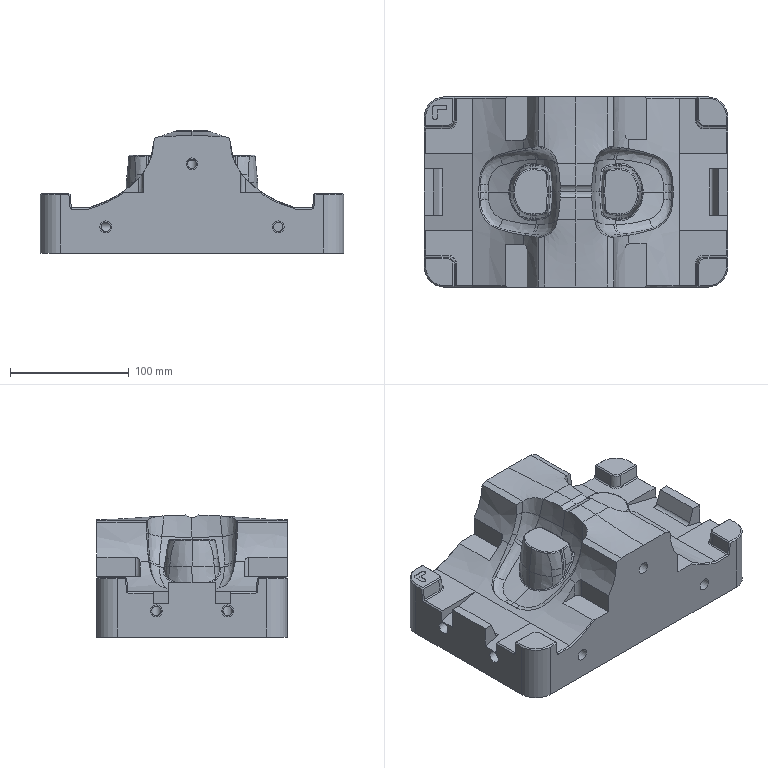NC program | NX | posted with a generic post | part box 255 x 160 x 102.619 mm
Lines 31654 to 32439 of 55104:
(ZLEVEL_PROFILE , TOOL : D8)
N63276 M6
N63278 G54
N63280 G17 G0 G90 X145.704 Y78.046 S3000 M3
N63282 G43 Z102.821 H0
N63284 G94 G1 Z102.321 F1800.
N63286 G3 X144.835 Y75.38 R4.
N63288 X145.715 Y64.863 R130.417
N63290 G1 X145.758 Y64.534 Z102.303
N63292 X145.803 Y64.205 Z102.286
N63294 X145.848 Y63.876 Z102.268
N63296 X145.894 Y63.547 Z102.25
N63298 X145.942 Y63.218 Z102.233
N63300 X145.99 Y62.889 Z102.215
N63302 X146.038 Y62.56 Z102.198
N63304 X146.139 Y61.903 Z102.163
N63306 X146.19 Y61.575 Z102.145
N63308 X146.243 Y61.246 Z102.127
N63310 X146.297 Y60.918 Z102.11
N63312 X146.351 Y60.59 Z102.092
N63314 X146.406 Y60.263 Z102.075
N63316 X146.463 Y59.935 Z102.057
N63318 X146.519 Y59.608 Z102.039
N63320 X146.576 Y59.28 Z102.022
N63322 G2 X144.847 Y75.699 R125.065
N63324 G1 X144.858 Y75.884 Z101.872
N63326 X144.854 Y76.068 Z101.723
N63328 G3 X146.596 Y59.289 R129.197
N63330 X147.378 Y55.437 R51.336
N63332 G1 Z103.723
N63334 G0 X147.537 Y97.962 Z102.821
N63336 G1 Z102.321
N63338 G3 X145.706 Y95.075 R4.
N63340 X144.836 Y84.633 R129.482
N63342 G1 X144.847 Y84.307 Z102.022
N63344 G2 X146.578 Y100.732 R124.772
N63346 G1 X146.636 Y101.053 Z101.997
N63348 X146.695 Y101.374 Z101.972
N63350 X146.755 Y101.694 Z101.947
N63352 X146.816 Y102.015 Z101.922
N63354 X146.878 Y102.336 Z101.897
N63356 X146.94 Y102.656 Z101.872
N63358 X147.005 Y102.976 Z101.847
N63360 X147.073 Y103.295 Z101.823
N63362 X147.144 Y103.614 Z101.798
N63364 X147.22 Y103.932 Z101.773
N63366 X147.3 Y104.248 Z101.748
N63368 X147.378 Y104.565 Z101.723
N63370 G3 X146.367 Y99.334 R63.16
N63372 G1 X146.151 Y97.953
N63374 G3 X144.853 Y83.935 R132.505
N63376 G1 Z103.723
N63378 G0 X150.199 Y51.086 Z101.924
N63380 G1 Z101.424
N63382 G2 X148.113 Y53.287 R4.
N63384 X147.001 Y57.217 R21.719
N63386 X144.87 Y76.489 R123.807
N63388 G3 X142.79 Y80.002 R4.184
N63390 X144.871 Y83.514 R4.196
N63392 G2 X147.001 Y102.786 R123.362
N63394 X148.115 Y106.72 R21.686
N63396 G1 X148.247 Y107.019 Z101.364
N63398 X148.381 Y107.318 Z101.304
N63400 X148.522 Y107.613 Z101.245
N63402 X148.67 Y107.906 Z101.185
N63404 X148.818 Y108.198 Z101.125
N63406 G3 X147.087 Y103.111 R19.726
N63408 X144.882 Y82.989 R123.078
N63410 G2 X143.554 Y80.002 R4.202
N63412 X144.882 Y77.009 R4.199
N63414 G3 X147.077 Y56.94 R123.912
N63416 X148.821 Y51.801 R19.921
N63418 G1 X148.985 Y51.522 Z101.05
N63420 X149.152 Y51.244 Z100.975
N63422 X149.327 Y50.97 Z100.901
N63424 X149.506 Y50.699 Z100.826
N63426 G2 X147.183 Y56.527 R16.935
N63428 X144.888 Y77.68 R123.758
N63430 G3 X144.196 Y80.002 R4.49
N63432 X144.888 Y82.321 R4.476
N63434 G2 X147.183 Y103.476 R123.252
N63436 X149.506 Y109.305 R16.932
N63438 G1 X149.664 Y109.523 Z100.751
N63440 X149.825 Y109.738 Z100.677
N63442 X149.992 Y109.95 Z100.602
N63444 X150.16 Y110.16 Z100.527
N63446 G3 X147.874 Y105.899 R13.8
N63448 X147.041 Y102.654 R25.809
N63450 X144.901 Y81.324 R124.227
N63452 G2 X144.753 Y80.002 R5.63
N63454 X144.901 Y78.679 R5.664
N63456 G3 X147.204 Y56.527 R123.237
N63458 X149.019 Y51.526 R17.978
N63460 X150.161 Y49.841 R10.25
N63462 G1 X150.377 Y49.605 Z100.427
N63464 X150.595 Y49.371 Z100.328
N63466 X150.817 Y49.141 Z100.228
N63468 G2 X148.571 Y52.428 R12.025
N63470 X147.179 Y56.771 R18.625
N63472 G1 X147.095 Y57.217
N63474 G2 X147.095 Y102.786 R121.14
N63476 G1 X147.141 Y103.029
N63478 G2 X148.309 Y106.987 R20.755
N63480 X150.817 Y110.863 R12.366
N63482 G1 X151.032 Y111.062 Z100.128
N63484 X151.249 Y111.259 Z100.029
N63486 X151.47 Y111.451 Z99.929
N63488 G3 X148.611 Y107.619 R11.659
N63490 X147.293 Y103.695 R19.539
N63492 X147.118 Y57.217 R121.302
N63494 G1 X147.188 Y56.841
N63496 G3 X148.599 Y52.41 R18.833
N63498 X151.47 Y48.552 R11.664
N63500 G1 X151.689 Y48.378 Z99.829
N63502 X151.91 Y48.208 Z99.73
N63504 X152.136 Y48.043 Z99.63
N63506 G2 X148.622 Y52.404 R11.441
N63508 X147.2 Y56.902 R18.959
N63510 G1 X147.142 Y57.217
N63512 G2 X146.973 Y101.869 R121.296
N63514 G1 X147.2 Y103.101
N63516 G2 X148.623 Y107.602 R18.929
N63518 X152.136 Y111.96 R11.447
N63520 G1 X152.348 Y112.105 Z99.53
N63522 X152.563 Y112.245 Z99.431
N63524 X152.78 Y112.382 Z99.331
N63526 G3 X148.673 Y107.666 R11.319
N63528 X147.29 Y103.476 R19.849
N63530 G1 X146.936 Y101.516
N63532 G3 X147.165 Y57.217 R121.39
N63534 G1 X147.293 Y56.511
N63536 G3 X148.673 Y52.338 R19.835
N63538 X152.776 Y47.624 R11.32
N63540 G1 X152.998 Y47.495 Z99.232
N63542 X153.222 Y47.37 Z99.132
N63544 X153.448 Y47.249 Z99.032
N63546 G2 X148.564 Y52.62 R11.269
N63548 X147.272 Y56.782 R20.026
N63550 X146.956 Y101.493 R121.596
N63552 G1 X147.246 Y103.106
N63554 G2 X148.676 Y107.632 R18.565
N63556 X153.445 Y112.752 R11.268
N63558 G1 X153.67 Y112.866 Z98.933
N63560 X153.898 Y112.976 Z98.833
N63562 X154.127 Y113.084 Z98.733
N63564 G3 X148.673 Y107.577 R11.28
N63566 X147.344 Y103.476 R18.726
N63568 X147.344 Y56.527 R122.248
N63570 X148.673 Y52.426 R19.026
N63572 X154.123 Y46.921 R11.279
N63574 G1 X154.355 Y46.822 Z98.634
N63576 X154.588 Y46.725 Z98.534
N63578 X154.821 Y46.629 Z98.434
N63580 G2 X148.673 Y52.476 R11.373
N63582 X147.372 Y56.527 R18.468
N63584 X147.372 Y103.476 R122.212
N63586 X148.673 Y107.527 R18.518
N63588 X154.818 Y113.373 R11.371
N63590 G1 Z100.434
N63592 G0 X159.396 Y162.579 Z98.635
N63594 G1 Z98.135
N63596 G3 X158.453 Y160.001 R4.
N63598 G1 X158.443 Y117.702
N63600 G2 X155.472 Y113.594 R4.327
N63602 G3 X148.673 Y107.477 R11.373
N63604 X147.399 Y103.476 R17.602
N63606 X147.4 Y56.527 R122.194
N63608 X149.709 Y50.694 R15.93
N63610 X155.365 Y46.445 R11.47
N63612 G2 X157.52 Y45. R5.05
N63614 X158.454 Y42.52 R3.759
N63616 G1 X158.453 Y0.002
N63618 X158.901 Z97.986
N63620 X159.346 Z97.836
N63622 X159.347 Y42.028
N63624 G3 X156.266 Y46.148 R4.19
N63626 G2 X153.704 Y47.201 R16.024
N63628 X149.137 Y51.675 R10.864
N63630 X147.427 Y56.527 R16.322
N63632 X147.427 Y103.476 R122.318
N63634 X148.77 Y107.619 R16.963
N63636 X152.063 Y111.761 R11.209
N63638 X156.266 Y113.849 R13.589
N63640 G3 X159.347 Y117.975 R4.205
N63642 G1 X159.346 Y160.001
N63644 X159.794 Z97.687
N63646 X160.24 Z97.537
N63648 X160.241 Y118.666
N63650 X160.24 Y117.975
N63652 G2 X156.956 Y114.025 R4.237
N63654 G3 X152.709 Y112.184 R14.04
N63656 X149.128 Y108.281 R10.542
N63658 X147.455 Y103.476 R16.685
N63660 X147.455 Y56.527 R122.482
N63662 X149.117 Y51.752 R16.366
N63664 X154.113 Y47.019 R10.863
N63666 X157.223 Y45.879 R19.541
N63668 G2 X160.24 Y41.929 R4.095
N63670 G1 Y0.002
N63672 X160.688 Z97.388
N63674 X161.134 Z97.238
N63676 X161.135 Y41.337
N63678 X161.126 Y42.028
N63680 G3 X157.668 Y45.825 R4.232
N63682 G2 X153.73 Y47.236 R15.521
N63684 X149.042 Y51.935 R10.962
N63686 X147.625 Y55.836 R16.256
N63688 G1 X147.342 Y57.217
N63690 G2 X147.482 Y103.476 R122.922
N63692 X149.118 Y108.212 R16.513
N63694 X153.054 Y112.377 R10.661
N63696 X157.68 Y114.178 R14.627
N63698 G3 X161.126 Y117.975 R4.245
N63700 G1 X161.135 Y118.666
N63702 X161.134 Y160.001
N63704 X161.582 Z97.089
N63706 X162.028 Z96.939
N63708 X162.029 Y118.666
N63710 X162.019 Y118.32
N63712 G2 X158.472 Y114.309 R4.183
N63714 G3 X153.043 Y112.347 R14.921
N63716 X149.168 Y108.258 R10.537
N63718 X147.51 Y103.476 R16.458
N63720 X147.51 Y56.527 R122.96
N63722 X149.083 Y51.907 R16.32
N63724 X153.808 Y47.218 R10.88
N63726 X158.523 Y45.676 R16.092
N63728 G2 X162.029 Y41.553 R4.177
N63730 G1 X162.028 Y0.002
N63732 X162.476 Z96.79
N63734 X162.915 Z96.64
N63736 X162.916 Y41.473
N63738 G3 X159.251 Y45.592 R4.147
N63740 G2 X153.844 Y47.222 R16.097
N63742 X149.088 Y51.949 R10.883
N63744 X147.538 Y56.527 R16.295
N63746 X147.538 Y103.476 R123.304
N63748 X149.164 Y108.206 R16.549
N63750 X153.067 Y112.337 R10.503
N63752 X158.336 Y114.271 R15.004
N63754 G1 X159.026 Y114.374
N63756 X159.533 Y114.464
N63758 G3 X162.916 Y118.505 R4.105
N63760 G1 X162.915 Y160.001
N63762 X163.018 Z96.603
N63764 X163.143 Z96.566
N63766 X163.184 Z96.528
N63768 X163.206 Z96.491
N63770 X163.22 Z96.342
N63772 X163.221 Y118.473
N63774 G2 X159.547 Y114.425 R4.067
N63776 G3 X153.538 Y112.591 R15.857
N63778 X149.149 Y108.127 R10.65
N63780 X147.565 Y103.476 R16.401
N63782 X147.566 Y56.527 R123.661
N63784 G1 X147.713 Y55.836
N63786 G3 X149.41 Y51.419 R14.926
N63788 X153.816 Y47.255 R10.683
N63790 X159.561 Y45.575 R16.266
N63792 G2 X163.221 Y41.532 R4.063
N63794 G1 X163.22 Y0.002
N63796 X163.24 Z96.043
N63798 Y41.542
N63800 G3 X159.568 Y45.593 R4.071
N63802 G2 X153.801 Y47.287 R16.104
N63804 X149.384 Y51.507 R10.715
N63806 X147.744 Y55.836 R14.786
N63808 G1 X147.593 Y56.527
N63810 G2 X147.593 Y103.476 R124.031
N63812 X148.922 Y107.619 R16.478
N63814 X153.962 Y112.797 R10.835
N63816 X159.567 Y114.41 R16.083
N63818 G3 X163.241 Y118.463 R4.072
N63820 G1 X163.24 Y160.001
N63822 X163.261 Z95.744
N63824 X163.262 Y118.451
N63826 G2 X159.581 Y114.396 R4.074
N63828 G3 X153.373 Y112.452 R15.824
N63830 X148.947 Y107.619 R10.749
N63832 X147.621 Y103.476 R17.174
N63834 G1 X147.251 Y101.375
N63836 G3 X147.499 Y57.217 R123.536
N63838 G1 X147.621 Y56.527
N63840 G3 X148.947 Y52.384 R17.143
N63842 X154.01 Y47.206 R10.831
N63844 X159.566 Y45.609 R16.14
N63846 G2 X163.261 Y41.524 R4.105
N63848 G1 X163.26 Y0.002
N63850 X163.282 Z95.445
N63852 X163.283 Y41.534
N63854 G3 X159.585 Y45.622 R4.109
N63856 G2 X154.059 Y47.206 R16.142
N63858 X148.972 Y52.384 R10.858
N63860 X147.651 Y56.527 R17.345
N63862 G1 X147.531 Y57.217
N63864 G2 X147.258 Y101.22 R123.691
N63866 G1 X147.651 Y103.476
N63868 G2 X148.972 Y107.619 R17.416
N63870 X153.417 Y112.452 R10.786
N63872 X159.603 Y114.383 R15.869
N63874 G3 X163.284 Y118.44 R4.076
N63876 G1 X163.283 Y160.001
N63878 X163.304 Z95.146
N63880 X163.306 Y118.427
N63882 G2 X159.626 Y114.37 R4.076
N63884 G3 X153.461 Y112.452 R15.91
N63886 X148.997 Y107.619 R10.827
N63888 X147.686 Y103.476 R17.336
N63890 X147.687 Y56.527 R124.646
N63892 X149.097 Y52.195 R16.412
N63894 X153.918 Y47.301 R10.798
N63896 X159.608 Y45.635 R16.161
N63898 G2 X163.305 Y41.547 R4.108
N63900 G1 X163.304 Y0.002
N63902 X163.326 Z94.847
N63904 X163.327 Y41.561
N63906 G3 X159.627 Y45.648 R4.107
N63908 G2 X153.607 Y47.495 R15.979
N63910 X149.197 Y52.05 R10.538
N63912 X147.722 Y56.527 R16.282
N63914 X147.721 Y103.476 R124.68
N63916 X149.024 Y107.619 R17.379
N63918 X153.505 Y112.452 R10.863
N63920 X159.626 Y114.355 R15.974
N63922 G3 X163.328 Y118.443 R4.109
N63924 G1 X163.326 Y160.001
N63926 X163.35 Z94.548
N63928 X163.352 Y118.431
N63930 G2 X159.651 Y114.342 R4.109
N63932 G3 X153.555 Y112.452 R15.957
N63934 X149.056 Y107.619 R10.792
N63936 X147.757 Y103.476 R16.978
N63938 X147.757 Y56.527 R124.676
N63940 G1 X147.9 Y55.836
N63942 G3 X149.364 Y51.785 R15.403
N63944 X153.85 Y47.399 R10.668
N63946 X159.648 Y45.661 R15.823
N63948 G2 X163.35 Y41.574 R4.107
N63950 G1 Y0.002
N63952 X163.377 Z94.249
N63954 Y41.614
N63956 G3 X159.704 Y45.672 R4.078
N63958 G2 X153.953 Y47.362 R16.184
N63960 X149.218 Y52.135 R10.772
N63962 X147.931 Y55.836 R15.189
N63964 X147.931 Y104.167 R124.532
N63966 X149.089 Y107.619 R16.017
N63968 X153.606 Y112.452 R10.732
N63970 X159.679 Y114.33 R15.995
N63972 G3 X163.378 Y118.419 R4.11
N63974 G1 X163.377 Y160.001
N63976 X163.403 Z93.95
N63978 X163.405 Y118.379
N63980 G2 X159.731 Y114.319 R4.079
N63982 G3 X153.657 Y112.452 R16.079
N63984 X149.122 Y107.619 R10.672
N63986 X147.962 Y104.167 R15.519
N63988 X147.962 Y55.836 R125.019
N63990 X149.48 Y51.694 R14.914
N63992 X154.195 Y47.269 R10.714
N63994 X159.73 Y45.685 R16.138
N63996 G2 X163.404 Y41.626 R4.079
N63998 G1 X163.403 Y0.002
N64000 X163.43 Z93.651
N64002 X163.431 Y41.637
N64004 G3 X159.753 Y45.699 R4.082
N64006 G2 X153.709 Y47.551 R16.046
N64008 X149.364 Y51.96 R10.647
N64010 X147.995 Y55.836 R15.525
N64012 X147.995 Y104.167 R125.489
N64014 X149.154 Y107.619 R15.665
N64016 X153.709 Y112.452 R10.63
N64018 X159.76 Y114.307 R16.126
N64020 G3 X163.432 Y118.366 R4.079
N64022 G1 X163.43 Y160.001
N64024 X163.457 Z93.352
N64026 X163.458 Y118.354
N64028 G2 X159.779 Y114.293 R4.08
N64030 G3 X153.505 Y112.301 R15.876
N64032 X149.187 Y107.619 R10.489
N64034 X148.033 Y104.167 R15.649
N64036 X148.033 Y55.836 R125.594
N64038 X149.364 Y52.018 R15.682
N64040 X153.505 Y47.702 R10.521
N64042 X159.773 Y45.713 R15.821
N64044 G2 X163.457 Y41.649 R4.083
N64046 G1 Y0.002
N64048 X163.483 Z93.053
N64050 X163.484 Y41.661
N64052 G3 X159.8 Y45.726 R4.084
N64054 G2 X153.505 Y47.732 R15.807
N64056 X149.182 Y52.458 R10.488
N64058 X148.02 Y56.074 R15.919
N64060 X148.071 Y104.167 R125.7
N64062 X149.219 Y107.619 R15.404
N64064 X153.505 Y112.271 R10.457
N64066 X159.805 Y114.28 R15.868
N64068 G3 X163.485 Y118.343 R4.082
N64070 G1 X163.483 Y160.001
N64072 X163.51 Z92.754
N64074 X163.512 Y118.331
N64076 G2 X159.831 Y114.267 R4.084
N64078 G3 X153.505 Y112.241 R15.859
N64080 X149.252 Y107.619 R10.457
N64082 X148.108 Y104.167 R15.197
N64084 X148.108 Y55.836 R125.772
N64086 X149.364 Y52.151 R15.212
N64088 X153.505 Y47.762 R10.474
N64090 X159.825 Y45.739 R15.784
N64092 G2 X163.511 Y41.673 R4.085
N64094 G1 X163.51 Y0.002
N64096 X163.526 Z92.604
N64098 X163.544 Z92.455
N64100 X163.545 Y41.673
N64102 G3 X159.852 Y45.752 R4.099
N64104 G2 X153.505 Y47.792 R15.86
N64106 X149.364 Y52.219 R10.476
N64108 X148.146 Y55.836 R15.109
N64110 X148.146 Y104.167 R126.035
N64112 X149.285 Y107.619 R15.143
N64114 X153.505 Y112.211 R10.471
N64116 X159.854 Y114.253 R15.886
N64118 G3 X163.545 Y118.333 R4.1
N64120 G1 X163.543 Y160.001
N64122 X163.557 Z92.306
N64124 X163.578 Z92.156
N64126 X163.58 Y118.332
N64128 G2 X159.889 Y114.241 R4.112
N64130 G3 X153.977 Y112.452 R16.243
N64132 X148.92 Y106.694 R10.676
N64134 X148.108 Y103.779 R18.437
N64136 X148.184 Y55.836 R126.328
N64138 X149.364 Y52.287 R15.083
N64140 X154.195 Y47.442 R10.613
N64142 X159.886 Y45.764 R16.096
N64144 G2 X163.579 Y41.676 R4.109
N64146 G1 X163.578 Y0.002
N64148 X163.587 Z92.007
N64150 X163.612 Z91.857
N64152 X163.613 Y41.681
N64154 G3 X159.91 Y45.777 R4.117
N64156 G2 X153.505 Y47.853 R15.959
N64158 X149.364 Y52.356 R10.523
N64160 X148.222 Y55.836 R15.368
N64162 X148.222 Y104.167 R126.564
N64164 X149.046 Y106.928 R16.204
N64166 X154.035 Y112.452 R10.64
N64168 X159.917 Y114.228 R16.264
N64170 G3 X163.614 Y118.328 R4.122
N64172 G1 X163.612 Y160.001
N64174 X163.62 Z91.708
N64176 X163.646 Z91.558
N64178 X163.648 Y118.318
N64180 G2 X159.952 Y114.216 R4.124
N64182 G3 X154.092 Y112.452 R16.345
N64184 X149.084 Y106.928 R10.597
N64186 X148.26 Y104.167 R16.18
N64188 X148.26 Y55.836 R127.01
N64190 X149.388 Y52.384 R15.423
N64192 X153.505 Y47.883 R10.5
N64194 X159.945 Y45.789 R16.032
N64196 G2 X163.647 Y41.691 R4.119
N64198 G1 X163.646 Y0.002
N64200 X163.653 Z91.409
N64202 X163.68 Z91.259
N64204 X163.681 Y41.701
N64206 G3 X159.979 Y45.802 R4.122
N64208 G2 X153.505 Y47.917 R16.059
N64210 X149.43 Y52.384 R10.381
N64212 X148.297 Y55.836 R15.182
N64214 X148.298 Y104.167 R127.353
N64216 X149.364 Y107.48 R15.382
N64218 X153.505 Y112.086 R10.408
N64220 X159.975 Y114.201 R16.057
N64222 G3 X163.682 Y118.307 R4.128
N64224 G1 X163.68 Y160.001
N64226 X163.687 Z91.11
N64228 X163.715 Z90.96
N64230 X163.716 Y118.297
N64232 G2 X160.001 Y114.184 R4.134
N64234 G3 X153.505 Y112.05 R15.965
N64236 X149.368 Y107.403 R10.307
N64238 X148.264 Y103.723 R14.917
N64240 G1 X148.223 Y103.476
N64242 X147.983 Y102.255
N64244 G3 X147.292 Y62.05 R128.354
N64246 G1 X147.831 Y58.665
N64248 G3 X148.224 Y56.527 R45.313
N64250 G1 X148.27 Y56.244
N64252 G3 X149.472 Y52.384 R14.465
N64254 X153.505 Y47.953 R10.258
N64256 X160.004 Y45.819 R15.962
N64258 G2 X163.715 Y41.711 R4.129
N64260 G1 X163.714 Y0.002
N64262 X163.722 Z90.811
N64264 X163.749 Z90.661
N64266 X163.75 Y41.721
N64268 G3 X160.032 Y45.835 R4.135
N64270 G2 X153.44 Y48.028 R15.917
N64272 X149.656 Y52.097 R10.037
N64274 X148.323 Y56.182 R14.071
N64276 G1 X148.267 Y56.527
N64278 G2 X146.147 Y75.859 R123.562
N64280 X147.883 Y101.405 R127.063
N64282 G1 X147.983 Y102.018
N64284 X148.266 Y103.476
N64286 X148.308 Y103.727
N64288 G2 X149.368 Y107.314 R15.068
N64290 X153.505 Y112.014 R10.262
N64292 X160.031 Y114.168 R15.92
N64294 G3 X163.75 Y118.286 R4.139
N64296 G1 X163.749 Y160.001
N64298 X163.758 Z90.512
N64300 X163.783 Z90.362
N64302 X163.785 Y118.241
N64304 G2 X160.163 Y114.185 R4.081
N64306 G3 X154.341 Y112.452 R17.294
N64308 X148.977 Y106.238 R10.632
N64310 X148.309 Y103.476 R18.112
N64312 G1 X148.178 Y102.786
N64314 G3 X148.044 Y57.908 R127.635
N64316 X148.673 Y54.778 R52.478
N64318 X151.434 Y49.664 R11.358
N64320 X154.885 Y47.284 R11.827
N64322 X160.163 Y45.818 R17.43
N64324 G2 X163.784 Y41.762 R4.082
N64326 G1 X163.783 Y0.002
N64328 X163.794 Z90.213
N64330 X163.817 Z90.063
N64332 X163.818 Y41.778
N64334 G3 X160.189 Y45.834 R4.081
N64336 G2 X154.026 Y47.754 R17.016
N64338 X149.564 Y52.44 R10.373
N64340 X148.488 Y55.78 R13.313
N64342 G1 X147.852 Y59.289
N64344 X147.753 Y59.979
N64346 X147.649 Y60.669
N64348 X147.54 Y61.36
N64350 G2 X148.091 Y102.095 R127.621
N64352 G1 X148.223 Y102.786
N64354 X148.353 Y103.476
N64356 X148.419 Y103.88
N64358 G2 X149.575 Y107.579 R13.966
N64360 X153.965 Y112.216 R10.279
N64362 X160.188 Y114.169 R16.995
N64364 G3 X163.819 Y118.226 R4.082
N64366 G1 X163.817 Y160.001
N64368 X163.832 Z89.914
N64370 X163.851 Z89.764
N64372 X163.853 Y118.207
N64374 G2 X160.218 Y114.152 R4.079
N64376 G3 X154.195 Y112.304 R16.772
N64378 X149.988 Y108.309 R10.455
N64380 X148.659 Y104.857 R13.462
N64382 X148.659 Y55.146 R127.419
N64384 X150.418 Y51.003 R12.767
N64386 X154.475 Y47.551 R10.83
N64388 X160.218 Y45.851 R16.854
N64390 G2 X163.852 Y41.796 R4.079
N64392 G1 X163.851 Y0.002
N64394 X163.871 Z89.615
N64396 X163.892 Z89.465
N64398 X163.885 Y41.834
N64400 G3 X160.265 Y45.864 R4.054
N64402 G2 X154.195 Y47.735 R16.675
N64404 X150.054 Y51.649 R10.391
N64406 X148.673 Y55.276 R13.43
N64408 X148.6 Y104.374 R127.731
N64410 X150.054 Y108.354 R13.432
N64412 X154.195 Y112.268 R10.374
N64414 X160.262 Y114.138 R16.612
N64416 G3 X163.889 Y118.131 R4.059
N64418 G1 X163.894 Y118.666
N64420 X163.893 Y160.001
N64422 X163.911 Z89.316
N64424 X163.935 Z89.166
N64426 X163.937 Y118.666
N64428 X163.932 Y118.158
N64430 G2 X160.273 Y114.12 R4.1
N64432 G3 X154.195 Y112.233 R16.567
N64434 X149.364 Y106.844 R10.402
N64436 X148.527 Y103.745 R16.284
N64438 G1 X148.482 Y103.476
N64440 X148.358 Y102.786
N64442 X148.232 Y102.095
N64444 G3 X148.482 Y56.527 R127.849
N64446 G1 X148.597 Y55.836
N64448 G3 X150.07 Y51.694 R13.954
N64450 X154.195 Y47.77 R10.356
N64452 X160.3 Y45.88 R16.583
N64454 G2 X163.926 Y41.846 R4.057
N64456 G1 X163.935 Y0.002
N64458 X163.951 Z89.017
N64460 X163.977 Z88.867
N64462 X163.968 Y41.83
N64464 G3 X160.316 Y45.897 R4.091
N64466 G2 X154.195 Y47.806 R16.58
N64468 X149.435 Y53.095 R10.219
N64470 X148.592 Y56.127 R14.854
N64472 G1 X148.525 Y56.527
N64474 G2 X148.403 Y102.786 R127.835
N64476 G1 X148.525 Y103.476
N64478 X148.593 Y103.884
N64480 G2 X149.436 Y106.911 R14.84
N64482 X154.195 Y112.198 R10.222
N64484 X160.308 Y114.105 R16.551
N64486 G3 X163.973 Y118.186 R4.106
N64488 G1 X163.978 Y160.001
N64490 X163.992 Z88.718
N64492 X164.02 Z88.568
N64494 X164.022 Y118.666
N64496 X164.018 Y118.145
N64498 G2 X160.347 Y114.09 R4.108
N64500 G3 X153.509 Y111.761 R16.433
N64502 X149.281 Y106.354 R10.109
N64504 X148.643 Y103.877 R19.618
N64506 X148.643 Y56.129 R128.596
N64508 X149.277 Y53.661 R19.721
N64510 X153.509 Y48.242 R10.111
N64512 X160.353 Y45.912 R16.447
N64514 G2 X164.01 Y41.844 R4.092
N64516 G1 X164.02 Y0.002
N64518 X164.035 Z88.419
N64520 X164.063 Z88.269
N64522 X164.053 Y41.859
N64524 G3 X160.395 Y45.926 R4.091
N64526 G2 X153.576 Y48.242 R16.404
N64528 X149.535 Y53.075 R10.007
N64530 X148.673 Y56.157 R16.947
N64532 G1 X148.612 Y56.527
N64534 G2 X148.372 Y102.095 R128.261
N64536 G1 X148.493 Y102.786
N64538 X148.611 Y103.476
N64540 G2 X149.364 Y106.49 R19.192
N64542 X154.195 Y112.127 R10.189
N64544 X160.394 Y114.076 R16.585
N64546 G3 X164.061 Y118.135 R4.108
N64548 G1 X164.064 Y118.666
N64550 X164.063 Y160.001
N64552 X164.078 Z88.12
N64554 X164.105 Z87.971
N64556 X164.107 Y118.666
N64558 X164.103 Y117.975
N64560 G2 X160.407 Y114.059 R4.109
N64562 G3 X154.195 Y112.09 R16.576
N64564 X149.146 Y105.64 R10.219
N64566 X148.642 Y103.358 R33.732
N64568 X148.787 Y55.836 R128.783
N64570 X149.581 Y53.075 R15.293
N64572 X153.643 Y48.242 R9.968
N64574 X160.435 Y45.941 R16.349
N64576 G2 X164.097 Y41.871 R4.093
N64578 G1 X164.105 Y0.002
N64580 X164.122 Z87.821
N64582 X164.148 Z87.672
N64584 X164.142 Y42.028
N64586 G3 X160.407 Y45.962 R4.096
N64588 G2 X153.711 Y48.242 R16.388
N64590 X149.627 Y53.075 R9.885
N64592 X148.838 Y55.836 R14.342
N64594 X148.466 Y102.095 R128.821
N64596 G1 X148.673 Y103.326
N64598 G2 X149.161 Y105.547 R29.33
N64600 X154.195 Y112.05 R10.202
N64602 X160.407 Y114.04 R16.553
N64604 G3 X164.146 Y117.975 R4.108
N64606 G1 X164.148 Y160.001
N64608 X164.167 Z87.522
N64610 X164.19 Z87.373
N64612 Y117.975
N64614 G2 X160.407 Y114.022 R4.103
N64616 G3 X154.195 Y112.01 R16.596
N64618 X149.205 Y105.547 R10.182
N64620 X148.673 Y103.056 R34.812
N64622 G1 X148.364 Y101.203
N64624 G3 X148.937 Y55.57 R128.98
N64626 X149.76 Y52.863 R13.53
N64628 X153.7 Y48.289 R9.86
N64630 X160.407 Y45.981 R16.458
N64632 G2 X164.188 Y42.028 R4.099
N64634 G1 X164.191 Y0.002
N64636 X164.214 Z87.223
N64638 X164.241 Z87.074
N64640 X164.24 Y41.895
N64642 G3 X160.573 Y45.981 R4.111
N64644 G2 X153.758 Y48.295 R16.55
N64646 X149.767 Y52.942 R9.895
N64648 X149.086 Y55.146 R12.088
N64650 G1 X148.94 Y55.836
N64652 G2 X148.568 Y102.141 R129.18
N64654 X149.179 Y105.248 R72.069
N64656 X152.815 Y111.056 R10.179
N64658 X160.555 Y114.019 R15.999
N64660 G3 X164.241 Y118.095 R4.111
N64662 G1 X164.242 Y118.666
N64664 X164.241 Y160.001
N64666 X164.263 Z86.924
N64668 X164.295 Z86.775
N64670 X164.294 Y118.113
N64672 G2 X160.61 Y114.005 R4.133
N64674 G3 X153.805 Y111.696 R16.581
N64676 X149.686 Y106.733 R9.88
N64678 X149.049 Y104.482 R13.802
N64680 X148.99 Y55.836 R129.202
N64682 G1 X149.134 Y55.146
N64684 G3 X149.708 Y53.201 R12.383
N64686 X153.813 Y48.302 R9.907
N64688 X160.611 Y45.998 R16.582
N64690 G2 X164.294 Y41.891 R4.131
N64692 G1 X164.295 Y0.002
N64694 X164.313 Z86.625
N64696 X164.349 Z86.476
N64698 X164.348 Y41.892
N64700 G3 X160.648 Y46.015 R4.147
N64702 G2 X153.505 Y48.542 R16.483
N64704 X150.054 Y52.503 R9.74
N64706 X149.182 Y55.146 R12.141
N64708 G1 X149.041 Y55.836
N64710 G2 X149.04 Y104.167 R129.32
N64712 G1 X149.18 Y104.857
N64714 G2 X149.918 Y107.191 R11.884
N64716 X153.567 Y111.501 R9.53
N64718 X160.647 Y113.988 R16.479
N64720 G3 X164.348 Y118.113 R4.149
N64722 G1 Y160.001
N64724 X164.366 Z86.326
N64726 X164.402 Z86.177
N64728 Y118.075
N64730 G2 X160.718 Y113.975 R4.124
N64732 G3 X153.505 Y111.419 R16.516
N64734 X149.608 Y106.238 R9.703
N64736 X149.228 Y104.857 R7.985
N64738 X149.092 Y55.836 R129.574
N64740 G1 X149.23 Y55.146
N64742 G3 X150.312 Y52.105 R11.049
N64744 X153.852 Y48.357 R9.721
N64746 X160.729 Y46.026 R16.737
N64748 G2 X164.402 Y41.933 R4.117
N64750 G1 Y0.002
N64752 X164.421 Z86.027
N64754 X164.456 Z85.878
N64756 Y41.97
N64758 G3 X160.843 Y46.016 R4.072
N64760 G2 X154.195 Y48.195 R17.303
N64762 X151.434 Y50.487 R10.601
N64764 X149.277 Y55.146 R10.736
N64766 X149.275 Y104.857 R129.704
N64768 X149.852 Y106.791 R12.829
N64770 X154.016 Y111.703 R9.797
N64772 X160.843 Y113.987 R17.277
N64774 G3 X164.456 Y118.033 R4.072
N64776 G1 Y160.001
N64778 X164.477 Z85.728
N64780 X164.51 Z85.579
N64782 Y118.004
N64784 G2 X160.902 Y113.969 R4.059
N64786 G3 X154.061 Y111.69 R17.286
N64788 X149.971 Y106.964 R9.765
N64790 X149.289 Y104.671 R12.175
N64792 X149.325 Y55.146 R130.111
N64794 X150.126 Y52.679 R11.477
N64796 X154.05 Y48.319 R9.746
N64798 X160.902 Y46.034 R17.296
N64800 G2 X164.51 Y42. R4.059
N64802 G1 X164.509 Y0.002
N64804 X164.536 Z85.429
N64806 X164.566 Z85.28
N64808 Y41.986
N64810 G3 X160.931 Y46.054 R4.093
N64812 G2 X154.195 Y48.282 R17.233
N64814 X150.303 Y52.384 R9.806
N64816 X149.364 Y55.2 R12.885
N64818 G1 X149.244 Y55.836
N64820 G2 X149.314 Y104.546 R130.46
N64822 X149.91 Y106.683 R13.427
N64824 X154.014 Y111.616 R9.641
N64826 X160.931 Y113.945 R17.273
N64828 G3 X164.567 Y117.975 R4.093
N64830 G1 Y160.001
N64832 X164.598 Z85.13
N64834 X164.633 Z84.981
N64836 X164.634 Y117.975
N64838 G2 X161.097 Y113.943 R4.105
N64840 G3 X153.505 Y111.223 R16.803